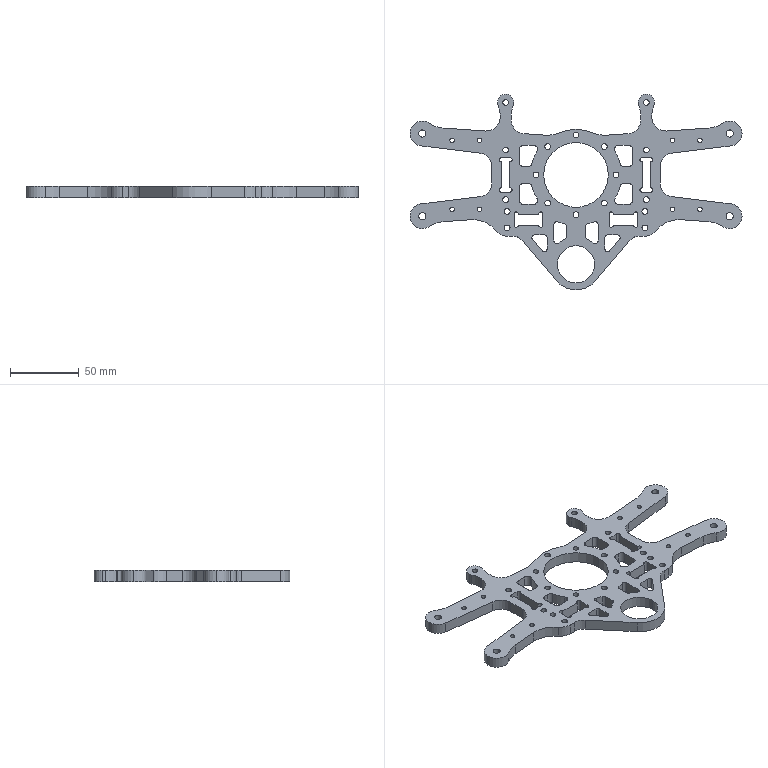Part | SolidWorks | features ICE 6, Fillet 3, Extrusion 1 | 1 solid | 223 faces | box 241 x 142.05 x 8 mm | volume 87619 mm3 | cylinder 163 | plane 60 | commonest cylinder face diameters 4.2 x36 6 x18 3.3 x16 4 x15 40 x14 3.2 x12